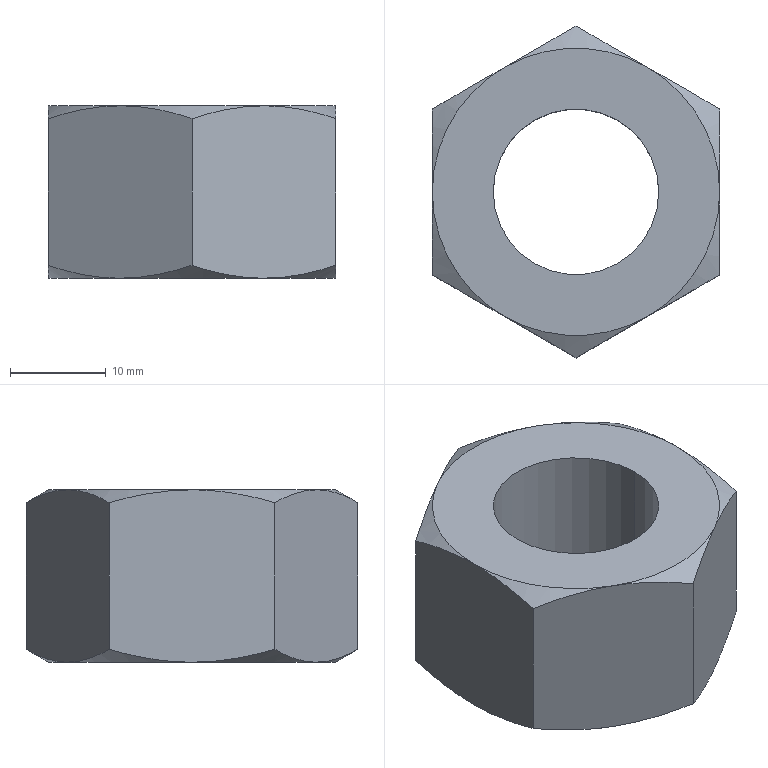Part | SolidWorks | features BaseBody 1 | 1 solid | 22 faces | box 30 x 34.641 x 18 mm | volume 9743 mm3 | cone 12 | plane 8 | cylinder 2 | commonest cylinder face diameters 17.294 x2
STEP:
#1=CARTESIAN_POINT('',(-8.647,0.,18.));
#2=VERTEX_POINT('',#1);
#3=CARTESIAN_POINT('',(8.647,0.,18.));
#4=VERTEX_POINT('',#3);
#5=CARTESIAN_POINT('',(0.,0.,18.));
#6=DIRECTION('',(0.,0.,1.));
#7=DIRECTION('',(1.,0.,0.));
#8=AXIS2_PLACEMENT_3D('',#5,#6,#7);
#9=CIRCLE('',#8,8.647);
#10=EDGE_CURVE('',#2,#4,#9,.T.);
#11=ORIENTED_EDGE('',*,*,#10,.T.);
#12=CARTESIAN_POINT('',(8.647,0.,0.));
#13=VERTEX_POINT('',#12);
#14=CARTESIAN_POINT('',(8.647,0.,18.));
#15=DIRECTION('',(0.,0.,-1.));
#16=VECTOR('',#15,1000.);
#17=LINE('',#14,#16);
#18=EDGE_CURVE('',#4,#13,#17,.T.);
#19=ORIENTED_EDGE('',*,*,#18,.T.);
#20=CARTESIAN_POINT('',(-8.647,0.,0.));
#21=VERTEX_POINT('',#20);
#22=CARTESIAN_POINT('',(0.,0.,0.));
#23=DIRECTION('',(0.,0.,1.));
#24=DIRECTION('',(1.,0.,0.));
#25=AXIS2_PLACEMENT_3D('',#22,#23,#24);
#26=CIRCLE('',#25,8.647);
#27=EDGE_CURVE('',#21,#13,#26,.T.);
#28=ORIENTED_EDGE('',*,*,#27,.F.);
#29=CARTESIAN_POINT('',(-8.647,0.,18.));
#30=DIRECTION('',(0.,0.,-1.));
#31=VECTOR('',#30,1000.);
#32=LINE('',#29,#31);
#33=EDGE_CURVE('',#2,#21,#32,.T.);
#34=ORIENTED_EDGE('',*,*,#33,.F.);
#35=EDGE_LOOP('',(#11,#19,#28,#34));
#36=FACE_OUTER_BOUND('',#35,.T.);
#37=CARTESIAN_POINT('',(0.,0.,18.));
#38=DIRECTION('',(0.,0.,-1.));
#39=DIRECTION('',(-1.,0.,0.));
#40=AXIS2_PLACEMENT_3D('',#37,#38,#39);
#41=CYLINDRICAL_SURFACE('',#40,8.647);
#42=ADVANCED_FACE('',(#36),#41,.F.);
#43=CARTESIAN_POINT('',(15.,8.66,16.66));
#44=VERTEX_POINT('',#43);
#45=CARTESIAN_POINT('',(7.5,12.99,18.));
#46=VERTEX_POINT('',#45);
#47=CARTESIAN_POINT('',(15.,8.66,16.66));
#48=CARTESIAN_POINT('',(13.773,9.369,17.069));
#49=CARTESIAN_POINT('',(12.537,10.082,17.406));
#50=CARTESIAN_POINT('',(10.04,11.524,17.872));
#51=CARTESIAN_POINT('',(8.778,12.253,18.));
#52=CARTESIAN_POINT('',(7.5,12.99,18.));
#53=B_SPLINE_CURVE_WITH_KNOTS('',3,(#47,#48,#49,#50,#51,#52),.UNSPECIFIED.,.F.,.F.,(4,2,4),(0.000000238,0.004382,0.008763),.UNSPECIFIED.);
#54=EDGE_CURVE('',#44,#46,#53,.T.);
#55=ORIENTED_EDGE('',*,*,#54,.F.);
#56=CARTESIAN_POINT('',(15.,8.66,1.34));
#57=VERTEX_POINT('',#56);
#58=CARTESIAN_POINT('',(15.,8.66,18.));
#59=DIRECTION('',(0.,0.,-1.));
#60=VECTOR('',#59,1000.);
#61=LINE('',#58,#60);
#62=EDGE_CURVE('',#44,#57,#61,.T.);
#63=ORIENTED_EDGE('',*,*,#62,.T.);
#64=CARTESIAN_POINT('',(7.5,12.99,0.));
#65=VERTEX_POINT('',#64);
#66=CARTESIAN_POINT('',(7.5,12.99,0.));
#67=CARTESIAN_POINT('',(8.136,12.623,0.));
#68=CARTESIAN_POINT('',(8.776,12.254,0.03167));
#69=CARTESIAN_POINT('',(10.041,11.524,0.1542));
#70=CARTESIAN_POINT('',(10.669,11.161,0.245));
#71=CARTESIAN_POINT('',(12.542,10.079,0.595));
#72=CARTESIAN_POINT('',(13.776,9.367,0.9318));
#73=CARTESIAN_POINT('',(15.,8.66,1.34));
#74=B_SPLINE_CURVE_WITH_KNOTS('',3,(#66,#67,#68,#69,#70,#71,#72,#73),.UNSPECIFIED.,.F.,.F.,(4,2,2,4),(0.008763,0.01095,0.01313,0.01749),.UNSPECIFIED.);
#75=EDGE_CURVE('',#65,#57,#74,.T.);
#76=ORIENTED_EDGE('',*,*,#75,.F.);
#77=CARTESIAN_POINT('',(0.,17.321,1.34));
#78=VERTEX_POINT('',#77);
#79=CARTESIAN_POINT('',(0.,17.321,1.34));
#80=CARTESIAN_POINT('',(1.227,16.612,0.9308));
#81=CARTESIAN_POINT('',(2.463,15.899,0.5939));
#82=CARTESIAN_POINT('',(4.96,14.457,0.1277));
#83=CARTESIAN_POINT('',(6.222,13.728,0.));
#84=CARTESIAN_POINT('',(7.5,12.99,0.));
#85=B_SPLINE_CURVE_WITH_KNOTS('',3,(#79,#80,#81,#82,#83,#84),.UNSPECIFIED.,.F.,.F.,(4,2,4),(0.000000238,0.004382,0.008763),.UNSPECIFIED.);
#86=EDGE_CURVE('',#78,#65,#85,.T.);
#87=ORIENTED_EDGE('',*,*,#86,.F.);
#88=CARTESIAN_POINT('',(0.,17.321,16.66));
#89=VERTEX_POINT('',#88);
#90=CARTESIAN_POINT('',(0.,17.321,18.));
#91=DIRECTION('',(0.,0.,-1.));
#92=VECTOR('',#91,1000.);
#93=LINE('',#90,#92);
#94=EDGE_CURVE('',#89,#78,#93,.T.);
#95=ORIENTED_EDGE('',*,*,#94,.F.);
#96=CARTESIAN_POINT('',(7.5,12.99,18.));
#97=CARTESIAN_POINT('',(6.864,13.358,18.));
#98=CARTESIAN_POINT('',(6.224,13.727,17.968));
#99=CARTESIAN_POINT('',(4.959,14.457,17.846));
#100=CARTESIAN_POINT('',(4.331,14.82,17.755));
#101=CARTESIAN_POINT('',(2.458,15.901,17.405));
#102=CARTESIAN_POINT('',(1.224,16.614,17.068));
#103=CARTESIAN_POINT('',(0.,17.321,16.66));
#104=B_SPLINE_CURVE_WITH_KNOTS('',3,(#96,#97,#98,#99,#100,#101,#102,#103),.UNSPECIFIED.,.F.,.F.,(4,2,2,4),(0.008763,0.01095,0.01313,0.01749),.UNSPECIFIED.);
#105=EDGE_CURVE('',#46,#89,#104,.T.);
#106=ORIENTED_EDGE('',*,*,#105,.F.);
#107=EDGE_LOOP('',(#55,#63,#76,#87,#95,#106));
#108=FACE_OUTER_BOUND('',#107,.T.);
#109=CARTESIAN_POINT('',(15.,8.66,18.));
#110=DIRECTION('',(-0.5,-0.866,0.));
#111=DIRECTION('',(0.866,-0.5,0.));
#112=AXIS2_PLACEMENT_3D('',#109,#110,#111);
#113=PLANE('',#112);
#114=ADVANCED_FACE('',(#108),#113,.F.);
#115=CARTESIAN_POINT('',(-7.5,12.99,18.));
#116=VERTEX_POINT('',#115);
#117=CARTESIAN_POINT('',(0.,17.321,16.66));
#118=CARTESIAN_POINT('',(-1.227,16.612,17.069));
#119=CARTESIAN_POINT('',(-2.463,15.899,17.406));
#120=CARTESIAN_POINT('',(-4.96,14.457,17.872));
#121=CARTESIAN_POINT('',(-6.222,13.728,18.));
#122=CARTESIAN_POINT('',(-7.5,12.99,18.));
#123=B_SPLINE_CURVE_WITH_KNOTS('',3,(#117,#118,#119,#120,#121,#122),.UNSPECIFIED.,.F.,.F.,(4,2,4),(0.000000238,0.004382,0.008763),.UNSPECIFIED.);
#124=EDGE_CURVE('',#89,#116,#123,.T.);
#125=ORIENTED_EDGE('',*,*,#124,.F.);
#126=ORIENTED_EDGE('',*,*,#94,.T.);
#127=CARTESIAN_POINT('',(-7.5,12.99,0.));
#128=VERTEX_POINT('',#127);
#129=CARTESIAN_POINT('',(-7.5,12.99,0.));
#130=CARTESIAN_POINT('',(-6.864,13.358,0.));
#131=CARTESIAN_POINT('',(-6.224,13.727,0.03167));
#132=CARTESIAN_POINT('',(-4.959,14.457,0.1542));
#133=CARTESIAN_POINT('',(-4.331,14.82,0.245));
#134=CARTESIAN_POINT('',(-2.458,15.901,0.595));
#135=CARTESIAN_POINT('',(-1.224,16.614,0.9318));
#136=CARTESIAN_POINT('',(0.,17.321,1.34));
#137=B_SPLINE_CURVE_WITH_KNOTS('',3,(#129,#130,#131,#132,#133,#134,#135,#136),.UNSPECIFIED.,.F.,.F.,(4,2,2,4),(0.008763,0.01095,0.01313,0.01749),.UNSPECIFIED.);
#138=EDGE_CURVE('',#128,#78,#137,.T.);
#139=ORIENTED_EDGE('',*,*,#138,.F.);
#140=CARTESIAN_POINT('',(-15.,8.66,1.34));
#141=VERTEX_POINT('',#140);
#142=CARTESIAN_POINT('',(-15.,8.66,1.34));
#143=CARTESIAN_POINT('',(-13.773,9.369,0.9308));
#144=CARTESIAN_POINT('',(-12.537,10.082,0.5939));
#145=CARTESIAN_POINT('',(-10.04,11.524,0.1277));
#146=CARTESIAN_POINT('',(-8.778,12.253,0.));
#147=CARTESIAN_POINT('',(-7.5,12.99,0.));
#148=B_SPLINE_CURVE_WITH_KNOTS('',3,(#142,#143,#144,#145,#146,#147),.UNSPECIFIED.,.F.,.F.,(4,2,4),(0.000000238,0.004382,0.008763),.UNSPECIFIED.);
#149=EDGE_CURVE('',#141,#128,#148,.T.);
#150=ORIENTED_EDGE('',*,*,#149,.F.);
#151=CARTESIAN_POINT('',(-15.,8.66,16.66));
#152=VERTEX_POINT('',#151);
#153=CARTESIAN_POINT('',(-15.,8.66,18.));
#154=DIRECTION('',(0.,0.,-1.));
#155=VECTOR('',#154,1000.);
#156=LINE('',#153,#155);
#157=EDGE_CURVE('',#152,#141,#156,.T.);
#158=ORIENTED_EDGE('',*,*,#157,.F.);
#159=CARTESIAN_POINT('',(-7.5,12.99,18.));
#160=CARTESIAN_POINT('',(-8.136,12.623,18.));
#161=CARTESIAN_POINT('',(-8.776,12.254,17.968));
#162=CARTESIAN_POINT('',(-10.041,11.524,17.846));
#163=CARTESIAN_POINT('',(-10.669,11.161,17.755));
#164=CARTESIAN_POINT('',(-12.542,10.079,17.405));
#165=CARTESIAN_POINT('',(-13.776,9.367,17.068));
#166=CARTESIAN_POINT('',(-15.,8.66,16.66));
#167=B_SPLINE_CURVE_WITH_KNOTS('',3,(#159,#160,#161,#162,#163,#164,#165,#166),.UNSPECIFIED.,.F.,.F.,(4,2,2,4),(0.008763,0.01095,0.01313,0.01749),.UNSPECIFIED.);
#168=EDGE_CURVE('',#116,#152,#167,.T.);
#169=ORIENTED_EDGE('',*,*,#168,.F.);
#170=EDGE_LOOP('',(#125,#126,#139,#150,#158,#169));
#171=FACE_OUTER_BOUND('',#170,.T.);
#172=CARTESIAN_POINT('',(0.,17.321,18.));
#173=DIRECTION('',(0.5,-0.866,0.));
#174=DIRECTION('',(0.866,0.5,0.));
#175=AXIS2_PLACEMENT_3D('',#172,#173,#174);
#176=PLANE('',#175);
#177=ADVANCED_FACE('',(#171),#176,.F.);
#178=CARTESIAN_POINT('',(-15.,0.,18.));
#179=VERTEX_POINT('',#178);
#180=CARTESIAN_POINT('',(-15.,8.66,16.66));
#181=CARTESIAN_POINT('',(-15.,7.26,17.065));
#182=CARTESIAN_POINT('',(-15.,5.841,17.401));
#183=CARTESIAN_POINT('',(-15.,3.673,17.753));
#184=CARTESIAN_POINT('',(-15.,2.944,17.845));
#185=CARTESIAN_POINT('',(-15.,1.469,17.969));
#186=CARTESIAN_POINT('',(-15.,0.7328,18.));
#187=CARTESIAN_POINT('',(-15.,0.,18.));
#188=B_SPLINE_CURVE_WITH_KNOTS('',3,(#180,#181,#182,#183,#184,#185,#186,#187),.UNSPECIFIED.,.F.,.F.,(4,2,2,4),(0.0493,0.05368,0.05587,0.05807),.UNSPECIFIED.);
#189=EDGE_CURVE('',#152,#179,#188,.T.);
#190=ORIENTED_EDGE('',*,*,#189,.F.);
#191=ORIENTED_EDGE('',*,*,#157,.T.);
#192=CARTESIAN_POINT('',(-15.,0.,0.));
#193=VERTEX_POINT('',#192);
#194=CARTESIAN_POINT('',(-15.,0.,0.));
#195=CARTESIAN_POINT('',(-15.,0.7328,0.));
#196=CARTESIAN_POINT('',(-15.,1.469,0.03124));
#197=CARTESIAN_POINT('',(-15.,2.944,0.1551));
#198=CARTESIAN_POINT('',(-15.,3.673,0.2469));
#199=CARTESIAN_POINT('',(-15.,5.841,0.5989));
#200=CARTESIAN_POINT('',(-15.,7.26,0.9354));
#201=CARTESIAN_POINT('',(-15.,8.66,1.34));
#202=B_SPLINE_CURVE_WITH_KNOTS('',3,(#194,#195,#196,#197,#198,#199,#200,#201),.UNSPECIFIED.,.F.,.F.,(4,2,2,4),(0.02463,0.02682,0.02901,0.0334),.UNSPECIFIED.);
#203=EDGE_CURVE('',#193,#141,#202,.T.);
#204=ORIENTED_EDGE('',*,*,#203,.F.);
#205=CARTESIAN_POINT('',(-15.,-8.66,1.34));
#206=VERTEX_POINT('',#205);
#207=CARTESIAN_POINT('',(-15.,-8.66,1.34));
#208=CARTESIAN_POINT('',(-15.,-7.251,0.9328));
#209=CARTESIAN_POINT('',(-15.,-5.808,0.592));
#210=CARTESIAN_POINT('',(-15.,-2.919,0.126));
#211=CARTESIAN_POINT('',(-15.,-1.465,0.));
#212=CARTESIAN_POINT('',(-15.,0.,0.));
#213=B_SPLINE_CURVE_WITH_KNOTS('',3,(#207,#208,#209,#210,#211,#212),.UNSPECIFIED.,.F.,.F.,(4,2,4),(0.01586,0.02025,0.02463),.UNSPECIFIED.);
#214=EDGE_CURVE('',#206,#193,#213,.T.);
#215=ORIENTED_EDGE('',*,*,#214,.F.);
#216=CARTESIAN_POINT('',(-15.,-8.66,16.66));
#217=VERTEX_POINT('',#216);
#218=CARTESIAN_POINT('',(-15.,-8.66,18.));
#219=DIRECTION('',(0.,0.,-1.));
#220=VECTOR('',#219,1000.);
#221=LINE('',#218,#220);
#222=EDGE_CURVE('',#217,#206,#221,.T.);
#223=ORIENTED_EDGE('',*,*,#222,.F.);
#224=CARTESIAN_POINT('',(-15.,0.,18.));
#225=CARTESIAN_POINT('',(-15.,-1.465,18.));
#226=CARTESIAN_POINT('',(-15.,-2.919,17.874));
#227=CARTESIAN_POINT('',(-15.,-5.808,17.408));
#228=CARTESIAN_POINT('',(-15.,-7.251,17.067));
#229=CARTESIAN_POINT('',(-15.,-8.66,16.66));
#230=B_SPLINE_CURVE_WITH_KNOTS('',3,(#224,#225,#226,#227,#228,#229),.UNSPECIFIED.,.F.,.F.,(4,2,4),(0.05807,0.06245,0.06683),.UNSPECIFIED.);
#231=EDGE_CURVE('',#179,#217,#230,.T.);
#232=ORIENTED_EDGE('',*,*,#231,.F.);
#233=EDGE_LOOP('',(#190,#191,#204,#215,#223,#232));
#234=FACE_OUTER_BOUND('',#233,.T.);
#235=CARTESIAN_POINT('',(-15.,8.66,18.));
#236=DIRECTION('',(1.,0.,0.));
#237=DIRECTION('',(0.,1.,0.));
#238=AXIS2_PLACEMENT_3D('',#235,#236,#237);
#239=PLANE('',#238);
#240=ADVANCED_FACE('',(#234),#239,.F.);
#241=CARTESIAN_POINT('',(-7.5,-12.99,18.));
#242=VERTEX_POINT('',#241);
#243=CARTESIAN_POINT('',(-15.,-8.66,16.66));
#244=CARTESIAN_POINT('',(-13.773,-9.369,17.069));
#245=CARTESIAN_POINT('',(-12.537,-10.082,17.406));
#246=CARTESIAN_POINT('',(-10.04,-11.524,17.872));
#247=CARTESIAN_POINT('',(-8.778,-12.253,18.));
#248=CARTESIAN_POINT('',(-7.5,-12.99,18.));
#249=B_SPLINE_CURVE_WITH_KNOTS('',3,(#243,#244,#245,#246,#247,#248),.UNSPECIFIED.,.F.,.F.,(4,2,4),(0.000000238,0.004382,0.008763),.UNSPECIFIED.);
#250=EDGE_CURVE('',#217,#242,#249,.T.);
#251=ORIENTED_EDGE('',*,*,#250,.F.);
#252=ORIENTED_EDGE('',*,*,#222,.T.);
#253=CARTESIAN_POINT('',(-7.5,-12.99,0.));
#254=VERTEX_POINT('',#253);
#255=CARTESIAN_POINT('',(-7.5,-12.99,0.));
#256=CARTESIAN_POINT('',(-8.136,-12.623,0.));
#257=CARTESIAN_POINT('',(-8.776,-12.254,0.03167));
#258=CARTESIAN_POINT('',(-10.041,-11.524,0.1542));
#259=CARTESIAN_POINT('',(-10.669,-11.161,0.245));
#260=CARTESIAN_POINT('',(-12.542,-10.079,0.595));
#261=CARTESIAN_POINT('',(-13.776,-9.367,0.9318));
#262=CARTESIAN_POINT('',(-15.,-8.66,1.34));
#263=B_SPLINE_CURVE_WITH_KNOTS('',3,(#255,#256,#257,#258,#259,#260,#261,#262),.UNSPECIFIED.,.F.,.F.,(4,2,2,4),(0.008763,0.01095,0.01313,0.01749),.UNSPECIFIED.);
#264=EDGE_CURVE('',#254,#206,#263,.T.);
#265=ORIENTED_EDGE('',*,*,#264,.F.);
#266=CARTESIAN_POINT('',(0.,-17.321,1.34));
#267=VERTEX_POINT('',#266);
#268=CARTESIAN_POINT('',(0.,-17.321,1.34));
#269=CARTESIAN_POINT('',(-1.227,-16.612,0.9308));
#270=CARTESIAN_POINT('',(-2.463,-15.899,0.5939));
#271=CARTESIAN_POINT('',(-4.96,-14.457,0.1277));
#272=CARTESIAN_POINT('',(-6.222,-13.728,0.));
#273=CARTESIAN_POINT('',(-7.5,-12.99,0.));
#274=B_SPLINE_CURVE_WITH_KNOTS('',3,(#268,#269,#270,#271,#272,#273),.UNSPECIFIED.,.F.,.F.,(4,2,4),(0.000000238,0.004382,0.008763),.UNSPECIFIED.);
#275=EDGE_CURVE('',#267,#254,#274,.T.);
#276=ORIENTED_EDGE('',*,*,#275,.F.);
#277=CARTESIAN_POINT('',(0.,-17.321,16.66));
#278=VERTEX_POINT('',#277);
#279=CARTESIAN_POINT('',(0.,-17.321,18.));
#280=DIRECTION('',(0.,0.,-1.));
#281=VECTOR('',#280,1000.);
#282=LINE('',#279,#281);
#283=EDGE_CURVE('',#278,#267,#282,.T.);
#284=ORIENTED_EDGE('',*,*,#283,.F.);
#285=CARTESIAN_POINT('',(-7.5,-12.99,18.));
#286=CARTESIAN_POINT('',(-6.864,-13.358,18.));
#287=CARTESIAN_POINT('',(-6.224,-13.727,17.968));
#288=CARTESIAN_POINT('',(-4.959,-14.457,17.846));
#289=CARTESIAN_POINT('',(-4.331,-14.82,17.755));
#290=CARTESIAN_POINT('',(-2.458,-15.901,17.405));
#291=CARTESIAN_POINT('',(-1.224,-16.614,17.068));
#292=CARTESIAN_POINT('',(0.,-17.321,16.66));
#293=B_SPLINE_CURVE_WITH_KNOTS('',3,(#285,#286,#287,#288,#289,#290,#291,#292),.UNSPECIFIED.,.F.,.F.,(4,2,2,4),(0.008763,0.01095,0.01313,0.01749),.UNSPECIFIED.);
#294=EDGE_CURVE('',#242,#278,#293,.T.);
#295=ORIENTED_EDGE('',*,*,#294,.F.);
#296=EDGE_LOOP('',(#251,#252,#265,#276,#284,#295));
#297=FACE_OUTER_BOUND('',#296,.T.);
#298=CARTESIAN_POINT('',(-15.,-8.66,18.));
#299=DIRECTION('',(0.5,0.866,0.));
#300=DIRECTION('',(-0.866,0.5,0.));
#301=AXIS2_PLACEMENT_3D('',#298,#299,#300);
#302=PLANE('',#301);
#303=ADVANCED_FACE('',(#297),#302,.F.);
#304=CARTESIAN_POINT('',(7.5,-12.99,18.));
#305=VERTEX_POINT('',#304);
#306=CARTESIAN_POINT('',(0.,-17.321,16.66));
#307=CARTESIAN_POINT('',(1.227,-16.612,17.069));
#308=CARTESIAN_POINT('',(2.463,-15.899,17.406));
#309=CARTESIAN_POINT('',(4.96,-14.457,17.872));
#310=CARTESIAN_POINT('',(6.222,-13.728,18.));
#311=CARTESIAN_POINT('',(7.5,-12.99,18.));
#312=B_SPLINE_CURVE_WITH_KNOTS('',3,(#306,#307,#308,#309,#310,#311),.UNSPECIFIED.,.F.,.F.,(4,2,4),(0.000000238,0.004382,0.008763),.UNSPECIFIED.);
#313=EDGE_CURVE('',#278,#305,#312,.T.);
#314=ORIENTED_EDGE('',*,*,#313,.F.);
#315=ORIENTED_EDGE('',*,*,#283,.T.);
#316=CARTESIAN_POINT('',(7.5,-12.99,0.));
#317=VERTEX_POINT('',#316);
#318=CARTESIAN_POINT('',(7.5,-12.99,0.));
#319=CARTESIAN_POINT('',(6.864,-13.358,0.));
#320=CARTESIAN_POINT('',(6.224,-13.727,0.03167));
#321=CARTESIAN_POINT('',(4.959,-14.457,0.1542));
#322=CARTESIAN_POINT('',(4.331,-14.82,0.245));
#323=CARTESIAN_POINT('',(2.458,-15.901,0.595));
#324=CARTESIAN_POINT('',(1.224,-16.614,0.9318));
#325=CARTESIAN_POINT('',(0.,-17.321,1.34));
#326=B_SPLINE_CURVE_WITH_KNOTS('',3,(#318,#319,#320,#321,#322,#323,#324,#325),.UNSPECIFIED.,.F.,.F.,(4,2,2,4),(0.008763,0.01095,0.01313,0.01749),.UNSPECIFIED.);
#327=EDGE_CURVE('',#317,#267,#326,.T.);
#328=ORIENTED_EDGE('',*,*,#327,.F.);
#329=CARTESIAN_POINT('',(15.,-8.66,1.34));
#330=VERTEX_POINT('',#329);
#331=CARTESIAN_POINT('',(15.,-8.66,1.34));
#332=CARTESIAN_POINT('',(13.773,-9.369,0.9308));
#333=CARTESIAN_POINT('',(12.537,-10.082,0.5939));
#334=CARTESIAN_POINT('',(10.04,-11.524,0.1277));
#335=CARTESIAN_POINT('',(8.778,-12.253,0.));
#336=CARTESIAN_POINT('',(7.5,-12.99,0.));
#337=B_SPLINE_CURVE_WITH_KNOTS('',3,(#331,#332,#333,#334,#335,#336),.UNSPECIFIED.,.F.,.F.,(4,2,4),(0.000000238,0.004382,0.008763),.UNSPECIFIED.);
#338=EDGE_CURVE('',#330,#317,#337,.T.);
#339=ORIENTED_EDGE('',*,*,#338,.F.);
#340=CARTESIAN_POINT('',(15.,-8.66,16.66));
#341=VERTEX_POINT('',#340);
#342=CARTESIAN_POINT('',(15.,-8.66,18.));
#343=DIRECTION('',(0.,0.,-1.));
#344=VECTOR('',#343,1000.);
#345=LINE('',#342,#344);
#346=EDGE_CURVE('',#341,#330,#345,.T.);
#347=ORIENTED_EDGE('',*,*,#346,.F.);
#348=CARTESIAN_POINT('',(7.5,-12.99,18.));
#349=CARTESIAN_POINT('',(8.136,-12.623,18.));
#350=CARTESIAN_POINT('',(8.776,-12.254,17.968));
#351=CARTESIAN_POINT('',(10.041,-11.524,17.846));
#352=CARTESIAN_POINT('',(10.669,-11.161,17.755));
#353=CARTESIAN_POINT('',(12.542,-10.079,17.405));
#354=CARTESIAN_POINT('',(13.776,-9.367,17.068));
#355=CARTESIAN_POINT('',(15.,-8.66,16.66));
#356=B_SPLINE_CURVE_WITH_KNOTS('',3,(#348,#349,#350,#351,#352,#353,#354,#355),.UNSPECIFIED.,.F.,.F.,(4,2,2,4),(0.008763,0.01095,0.01313,0.01749),.UNSPECIFIED.);
#357=EDGE_CURVE('',#305,#341,#356,.T.);
#358=ORIENTED_EDGE('',*,*,#357,.F.);
#359=EDGE_LOOP('',(#314,#315,#328,#339,#347,#358));
#360=FACE_OUTER_BOUND('',#359,.T.);
#361=CARTESIAN_POINT('',(0.,-17.321,18.));
#362=DIRECTION('',(-0.5,0.866,0.));
#363=DIRECTION('',(-0.866,-0.5,0.));
#364=AXIS2_PLACEMENT_3D('',#361,#362,#363);
#365=PLANE('',#364);
#366=ADVANCED_FACE('',(#360),#365,.F.);
#367=CARTESIAN_POINT('',(15.,0.,18.));
#368=VERTEX_POINT('',#367);
#369=CARTESIAN_POINT('',(15.,-8.66,16.66));
#370=CARTESIAN_POINT('',(15.,-7.251,17.067));
#371=CARTESIAN_POINT('',(15.,-5.808,17.408));
#372=CARTESIAN_POINT('',(15.,-2.919,17.874));
#373=CARTESIAN_POINT('',(15.,-1.465,18.));
#374=CARTESIAN_POINT('',(15.,0.,18.));
#375=B_SPLINE_CURVE_WITH_KNOTS('',3,(#369,#370,#371,#372,#373,#374),.UNSPECIFIED.,.F.,.F.,(4,2,4),(0.01586,0.02025,0.02463),.UNSPECIFIED.);
#376=EDGE_CURVE('',#341,#368,#375,.T.);
#377=ORIENTED_EDGE('',*,*,#376,.F.);
#378=ORIENTED_EDGE('',*,*,#346,.T.);
#379=CARTESIAN_POINT('',(15.,0.,0.));
#380=VERTEX_POINT('',#379);
#381=CARTESIAN_POINT('',(15.,0.,0.));
#382=CARTESIAN_POINT('',(15.,-1.465,0.));
#383=CARTESIAN_POINT('',(15.,-2.919,0.126));
#384=CARTESIAN_POINT('',(15.,-5.808,0.592));
#385=CARTESIAN_POINT('',(15.,-7.251,0.9328));
#386=CARTESIAN_POINT('',(15.,-8.66,1.34));
#387=B_SPLINE_CURVE_WITH_KNOTS('',3,(#381,#382,#383,#384,#385,#386),.UNSPECIFIED.,.F.,.F.,(4,2,4),(0.05807,0.06245,0.06683),.UNSPECIFIED.);
#388=EDGE_CURVE('',#380,#330,#387,.T.);
#389=ORIENTED_EDGE('',*,*,#388,.F.);
#390=CARTESIAN_POINT('',(15.,8.66,1.34));
#391=CARTESIAN_POINT('',(15.,7.26,0.9354));
#392=CARTESIAN_POINT('',(15.,5.841,0.5989));
#393=CARTESIAN_POINT('',(15.,3.673,0.2469));
#394=CARTESIAN_POINT('',(15.,2.944,0.1551));
#395=CARTESIAN_POINT('',(15.,1.469,0.03124));
#396=CARTESIAN_POINT('',(15.,0.7328,0.));
#397=CARTESIAN_POINT('',(15.,0.,0.));
#398=B_SPLINE_CURVE_WITH_KNOTS('',3,(#390,#391,#392,#393,#394,#395,#396,#397),.UNSPECIFIED.,.F.,.F.,(4,2,2,4),(0.0493,0.05368,0.05587,0.05807),.UNSPECIFIED.);
#399=EDGE_CURVE('',#57,#380,#398,.T.);
#400=ORIENTED_EDGE('',*,*,#399,.F.);
#401=ORIENTED_EDGE('',*,*,#62,.F.);
#402=CARTESIAN_POINT('',(15.,0.,18.));
#403=CARTESIAN_POINT('',(15.,0.7328,18.));
#404=CARTESIAN_POINT('',(15.,1.469,17.969));
#405=CARTESIAN_POINT('',(15.,2.944,17.845));
#406=CARTESIAN_POINT('',(15.,3.673,17.753));
#407=CARTESIAN_POINT('',(15.,5.841,17.401));
#408=CARTESIAN_POINT('',(15.,7.26,17.065));
#409=CARTESIAN_POINT('',(15.,8.66,16.66));
#410=B_SPLINE_CURVE_WITH_KNOTS('',3,(#402,#403,#404,#405,#406,#407,#408,#409),.UNSPECIFIED.,.F.,.F.,(4,2,2,4),(0.02463,0.02682,0.02901,0.0334),.UNSPECIFIED.);
#411=EDGE_CURVE('',#368,#44,#410,.T.);
#412=ORIENTED_EDGE('',*,*,#411,.F.);
#413=EDGE_LOOP('',(#377,#378,#389,#400,#401,#412));
#414=FACE_OUTER_BOUND('',#413,.T.);
#415=CARTESIAN_POINT('',(15.,-8.66,18.));
#416=DIRECTION('',(-1.,0.,0.));
#417=DIRECTION('',(0.,-1.,0.));
#418=AXIS2_PLACEMENT_3D('',#415,#416,#417);
#419=PLANE('',#418);
#420=ADVANCED_FACE('',(#414),#419,.F.);
#421=ORIENTED_EDGE('',*,*,#10,.F.);
#422=CARTESIAN_POINT('',(0.,0.,18.));
#423=DIRECTION('',(0.,0.,1.));
#424=DIRECTION('',(1.,0.,0.));
#425=AXIS2_PLACEMENT_3D('',#422,#423,#424);
#426=CIRCLE('',#425,8.647);
#427=EDGE_CURVE('',#4,#2,#426,.T.);
#428=ORIENTED_EDGE('',*,*,#427,.F.);
#429=EDGE_LOOP('',(#421,#428));
#430=FACE_BOUND('',#429,.T.);
#431=CARTESIAN_POINT('',(0.,0.,18.));
#432=DIRECTION('',(0.,0.,1.));
#433=DIRECTION('',(1.,0.,0.));
#434=AXIS2_PLACEMENT_3D('',#431,#432,#433);
#435=CIRCLE('',#434,15.);
#436=EDGE_CURVE('',#305,#368,#435,.T.);
#437=ORIENTED_EDGE('',*,*,#436,.T.);
#438=CARTESIAN_POINT('',(0.,0.,18.));
#439=DIRECTION('',(0.,0.,1.));
#440=DIRECTION('',(1.,0.,0.));
#441=AXIS2_PLACEMENT_3D('',#438,#439,#440);
#442=CIRCLE('',#441,15.);
#443=EDGE_CURVE('',#368,#46,#442,.T.);
#444=ORIENTED_EDGE('',*,*,#443,.T.);
#445=CARTESIAN_POINT('',(0.,0.,18.));
#446=DIRECTION('',(0.,0.,1.));
#447=DIRECTION('',(1.,0.,0.));
#448=AXIS2_PLACEMENT_3D('',#445,#446,#447);
#449=CIRCLE('',#448,15.);
#450=EDGE_CURVE('',#46,#116,#449,.T.);
#451=ORIENTED_EDGE('',*,*,#450,.T.);
#452=CARTESIAN_POINT('',(0.,0.,18.));
#453=DIRECTION('',(0.,0.,1.));
#454=DIRECTION('',(1.,0.,0.));
#455=AXIS2_PLACEMENT_3D('',#452,#453,#454);
#456=CIRCLE('',#455,15.);
#457=EDGE_CURVE('',#116,#179,#456,.T.);
#458=ORIENTED_EDGE('',*,*,#457,.T.);
#459=CARTESIAN_POINT('',(0.,0.,18.));
#460=DIRECTION('',(0.,0.,1.));
#461=DIRECTION('',(1.,0.,0.));
#462=AXIS2_PLACEMENT_3D('',#459,#460,#461);
#463=CIRCLE('',#462,15.);
#464=EDGE_CURVE('',#179,#242,#463,.T.);
#465=ORIENTED_EDGE('',*,*,#464,.T.);
#466=CARTESIAN_POINT('',(0.,0.,18.));
#467=DIRECTION('',(0.,0.,1.));
#468=DIRECTION('',(1.,0.,0.));
#469=AXIS2_PLACEMENT_3D('',#466,#467,#468);
#470=CIRCLE('',#469,15.);
#471=EDGE_CURVE('',#242,#305,#470,.T.);
#472=ORIENTED_EDGE('',*,*,#471,.T.);
#473=EDGE_LOOP('',(#437,#444,#451,#458,#465,#472));
#474=FACE_OUTER_BOUND('',#473,.T.);
#475=CARTESIAN_POINT('',(-15.,25.981,18.));
#476=DIRECTION('',(0.,0.,1.));
#477=DIRECTION('',(1.,0.,0.));
#478=AXIS2_PLACEMENT_3D('',#475,#476,#477);
#479=PLANE('',#478);
#480=ADVANCED_FACE('',(#430,#474),#479,.T.);
#481=ORIENTED_EDGE('',*,*,#27,.T.);
#482=CARTESIAN_POINT('',(0.,0.,0.));
#483=DIRECTION('',(0.,0.,1.));
#484=DIRECTION('',(1.,0.,0.));
#485=AXIS2_PLACEMENT_3D('',#482,#483,#484);
#486=CIRCLE('',#485,8.647);
#487=EDGE_CURVE('',#13,#21,#486,.T.);
#488=ORIENTED_EDGE('',*,*,#487,.T.);
#489=EDGE_LOOP('',(#481,#488));
#490=FACE_BOUND('',#489,.T.);
#491=CARTESIAN_POINT('',(0.,0.,0.));
#492=DIRECTION('',(0.,0.,-1.));
#493=DIRECTION('',(-1.,0.,0.));
#494=AXIS2_PLACEMENT_3D('',#491,#492,#493);
#495=CIRCLE('',#494,15.);
#496=EDGE_CURVE('',#65,#380,#495,.T.);
#497=ORIENTED_EDGE('',*,*,#496,.T.);
#498=CARTESIAN_POINT('',(0.,0.,0.));
#499=DIRECTION('',(0.,0.,-1.));
#500=DIRECTION('',(-1.,0.,0.));
#501=AXIS2_PLACEMENT_3D('',#498,#499,#500);
#502=CIRCLE('',#501,15.);
#503=EDGE_CURVE('',#380,#317,#502,.T.);
#504=ORIENTED_EDGE('',*,*,#503,.T.);
#505=CARTESIAN_POINT('',(0.,0.,0.));
#506=DIRECTION('',(0.,0.,-1.));
#507=DIRECTION('',(-1.,0.,0.));
#508=AXIS2_PLACEMENT_3D('',#505,#506,#507);
#509=CIRCLE('',#508,15.);
#510=EDGE_CURVE('',#317,#254,#509,.T.);
#511=ORIENTED_EDGE('',*,*,#510,.T.);
#512=CARTESIAN_POINT('',(0.,0.,0.));
#513=DIRECTION('',(0.,0.,-1.));
#514=DIRECTION('',(-1.,0.,0.));
#515=AXIS2_PLACEMENT_3D('',#512,#513,#514);
#516=CIRCLE('',#515,15.);
#517=EDGE_CURVE('',#254,#193,#516,.T.);
#518=ORIENTED_EDGE('',*,*,#517,.T.);
#519=CARTESIAN_POINT('',(0.,0.,0.));
#520=DIRECTION('',(0.,0.,-1.));
#521=DIRECTION('',(-1.,0.,0.));
#522=AXIS2_PLACEMENT_3D('',#519,#520,#521);
#523=CIRCLE('',#522,15.);
#524=EDGE_CURVE('',#193,#128,#523,.T.);
#525=ORIENTED_EDGE('',*,*,#524,.T.);
#526=CARTESIAN_POINT('',(0.,0.,0.));
#527=DIRECTION('',(0.,0.,-1.));
#528=DIRECTION('',(-1.,0.,0.));
#529=AXIS2_PLACEMENT_3D('',#526,#527,#528);
#530=CIRCLE('',#529,15.);
#531=EDGE_CURVE('',#128,#65,#530,.T.);
#532=ORIENTED_EDGE('',*,*,#531,.T.);
#533=EDGE_LOOP('',(#497,#504,#511,#518,#525,#532));
#534=FACE_OUTER_BOUND('',#533,.T.);
#535=CARTESIAN_POINT('',(-15.,25.981,0.));
#536=DIRECTION('',(0.,0.,1.));
#537=DIRECTION('',(1.,0.,0.));
#538=AXIS2_PLACEMENT_3D('',#535,#536,#537);
#539=PLANE('',#538);
#540=ADVANCED_FACE('',(#490,#534),#539,.F.);
#541=ORIENTED_EDGE('',*,*,#18,.F.);
#542=ORIENTED_EDGE('',*,*,#427,.T.);
#543=ORIENTED_EDGE('',*,*,#33,.T.);
#544=ORIENTED_EDGE('',*,*,#487,.F.);
#545=EDGE_LOOP('',(#541,#542,#543,#544));
#546=FACE_OUTER_BOUND('',#545,.T.);
#547=CARTESIAN_POINT('',(0.,0.,18.));
#548=DIRECTION('',(0.,0.,-1.));
#549=DIRECTION('',(-1.,0.,0.));
#550=AXIS2_PLACEMENT_3D('',#547,#548,#549);
#551=CYLINDRICAL_SURFACE('',#550,8.647);
#552=ADVANCED_FACE('',(#546),#551,.F.);
#553=ORIENTED_EDGE('',*,*,#338,.T.);
#554=ORIENTED_EDGE('',*,*,#503,.F.);
#555=ORIENTED_EDGE('',*,*,#388,.T.);
#556=EDGE_LOOP('',(#553,#554,#555));
#557=FACE_OUTER_BOUND('',#556,.T.);
#558=CARTESIAN_POINT('',(0.,0.,0.));
#559=DIRECTION('',(0.,0.,1.));
#560=DIRECTION('',(-1.,0.,0.));
#561=AXIS2_PLACEMENT_3D('',#558,#559,#560);
#562=CONICAL_SURFACE('',#561,15.,1.047);
#563=ADVANCED_FACE('',(#557),#562,.T.);
#564=ORIENTED_EDGE('',*,*,#75,.T.);
#565=ORIENTED_EDGE('',*,*,#399,.T.);
#566=ORIENTED_EDGE('',*,*,#496,.F.);
#567=EDGE_LOOP('',(#564,#565,#566));
#568=FACE_OUTER_BOUND('',#567,.T.);
#569=CARTESIAN_POINT('',(0.,0.,0.));
#570=DIRECTION('',(0.,0.,1.));
#571=DIRECTION('',(-1.,0.,0.));
#572=AXIS2_PLACEMENT_3D('',#569,#570,#571);
#573=CONICAL_SURFACE('',#572,15.,1.047);
#574=ADVANCED_FACE('',(#568),#573,.T.);
#575=ORIENTED_EDGE('',*,*,#275,.T.);
#576=ORIENTED_EDGE('',*,*,#510,.F.);
#577=ORIENTED_EDGE('',*,*,#327,.T.);
#578=EDGE_LOOP('',(#575,#576,#577));
#579=FACE_OUTER_BOUND('',#578,.T.);
#580=CARTESIAN_POINT('',(0.,0.,0.));
#581=DIRECTION('',(0.,0.,1.));
#582=DIRECTION('',(-1.,0.,0.));
#583=AXIS2_PLACEMENT_3D('',#580,#581,#582);
#584=CONICAL_SURFACE('',#583,15.,1.047);
#585=ADVANCED_FACE('',(#579),#584,.T.);
#586=ORIENTED_EDGE('',*,*,#214,.T.);
#587=ORIENTED_EDGE('',*,*,#517,.F.);
#588=ORIENTED_EDGE('',*,*,#264,.T.);
#589=EDGE_LOOP('',(#586,#587,#588));
#590=FACE_OUTER_BOUND('',#589,.T.);
#591=CARTESIAN_POINT('',(0.,0.,0.));
#592=DIRECTION('',(0.,0.,1.));
#593=DIRECTION('',(-1.,0.,0.));
#594=AXIS2_PLACEMENT_3D('',#591,#592,#593);
#595=CONICAL_SURFACE('',#594,15.,1.047);
#596=ADVANCED_FACE('',(#590),#595,.T.);
#597=ORIENTED_EDGE('',*,*,#203,.T.);
#598=ORIENTED_EDGE('',*,*,#149,.T.);
#599=ORIENTED_EDGE('',*,*,#524,.F.);
#600=EDGE_LOOP('',(#597,#598,#599));
#601=FACE_OUTER_BOUND('',#600,.T.);
#602=CARTESIAN_POINT('',(0.,0.,0.));
#603=DIRECTION('',(0.,0.,1.));
#604=DIRECTION('',(-1.,0.,0.));
#605=AXIS2_PLACEMENT_3D('',#602,#603,#604);
#606=CONICAL_SURFACE('',#605,15.,1.047);
#607=ADVANCED_FACE('',(#601),#606,.T.);
#608=ORIENTED_EDGE('',*,*,#138,.T.);
#609=ORIENTED_EDGE('',*,*,#86,.T.);
#610=ORIENTED_EDGE('',*,*,#531,.F.);
#611=EDGE_LOOP('',(#608,#609,#610));
#612=FACE_OUTER_BOUND('',#611,.T.);
#613=CARTESIAN_POINT('',(0.,0.,0.));
#614=DIRECTION('',(0.,0.,1.));
#615=DIRECTION('',(-1.,0.,0.));
#616=AXIS2_PLACEMENT_3D('',#613,#614,#615);
#617=CONICAL_SURFACE('',#616,15.,1.047);
#618=ADVANCED_FACE('',(#612),#617,.T.);
#619=ORIENTED_EDGE('',*,*,#357,.T.);
#620=ORIENTED_EDGE('',*,*,#376,.T.);
#621=ORIENTED_EDGE('',*,*,#436,.F.);
#622=EDGE_LOOP('',(#619,#620,#621));
#623=FACE_OUTER_BOUND('',#622,.T.);
#624=CARTESIAN_POINT('',(0.,0.,18.));
#625=DIRECTION('',(0.,0.,-1.));
#626=DIRECTION('',(1.,0.,0.));
#627=AXIS2_PLACEMENT_3D('',#624,#625,#626);
#628=CONICAL_SURFACE('',#627,15.,1.047);
#629=ADVANCED_FACE('',(#623),#628,.T.);
#630=ORIENTED_EDGE('',*,*,#294,.T.);
#631=ORIENTED_EDGE('',*,*,#313,.T.);
#632=ORIENTED_EDGE('',*,*,#471,.F.);
#633=EDGE_LOOP('',(#630,#631,#632));
#634=FACE_OUTER_BOUND('',#633,.T.);
#635=CARTESIAN_POINT('',(0.,0.,18.));
#636=DIRECTION('',(0.,0.,-1.));
#637=DIRECTION('',(1.,0.,0.));
#638=AXIS2_PLACEMENT_3D('',#635,#636,#637);
#639=CONICAL_SURFACE('',#638,15.,1.047);
#640=ADVANCED_FACE('',(#634),#639,.T.);
#641=ORIENTED_EDGE('',*,*,#231,.T.);
#642=ORIENTED_EDGE('',*,*,#250,.T.);
#643=ORIENTED_EDGE('',*,*,#464,.F.);
#644=EDGE_LOOP('',(#641,#642,#643));
#645=FACE_OUTER_BOUND('',#644,.T.);
#646=CARTESIAN_POINT('',(0.,0.,18.));
#647=DIRECTION('',(0.,0.,-1.));
#648=DIRECTION('',(1.,0.,0.));
#649=AXIS2_PLACEMENT_3D('',#646,#647,#648);
#650=CONICAL_SURFACE('',#649,15.,1.047);
#651=ADVANCED_FACE('',(#645),#650,.T.);
#652=ORIENTED_EDGE('',*,*,#168,.T.);
#653=ORIENTED_EDGE('',*,*,#189,.T.);
#654=ORIENTED_EDGE('',*,*,#457,.F.);
#655=EDGE_LOOP('',(#652,#653,#654));
#656=FACE_OUTER_BOUND('',#655,.T.);
#657=CARTESIAN_POINT('',(0.,0.,18.));
#658=DIRECTION('',(0.,0.,-1.));
#659=DIRECTION('',(1.,0.,0.));
#660=AXIS2_PLACEMENT_3D('',#657,#658,#659);
#661=CONICAL_SURFACE('',#660,15.,1.047);
#662=ADVANCED_FACE('',(#656),#661,.T.);
#663=ORIENTED_EDGE('',*,*,#105,.T.);
#664=ORIENTED_EDGE('',*,*,#124,.T.);
#665=ORIENTED_EDGE('',*,*,#450,.F.);
#666=EDGE_LOOP('',(#663,#664,#665));
#667=FACE_OUTER_BOUND('',#666,.T.);
#668=CARTESIAN_POINT('',(0.,0.,18.));
#669=DIRECTION('',(0.,0.,-1.));
#670=DIRECTION('',(1.,0.,0.));
#671=AXIS2_PLACEMENT_3D('',#668,#669,#670);
#672=CONICAL_SURFACE('',#671,15.,1.047);
#673=ADVANCED_FACE('',(#667),#672,.T.);
#674=ORIENTED_EDGE('',*,*,#54,.T.);
#675=ORIENTED_EDGE('',*,*,#443,.F.);
#676=ORIENTED_EDGE('',*,*,#411,.T.);
#677=EDGE_LOOP('',(#674,#675,#676));
#678=FACE_OUTER_BOUND('',#677,.T.);
#679=CARTESIAN_POINT('',(0.,0.,18.));
#680=DIRECTION('',(0.,0.,-1.));
#681=DIRECTION('',(1.,0.,0.));
#682=AXIS2_PLACEMENT_3D('',#679,#680,#681);
#683=CONICAL_SURFACE('',#682,15.,1.047);
#684=ADVANCED_FACE('',(#678),#683,.T.);
#685=CLOSED_SHELL('',(#42,#114,#177,#240,#303,#366,#420,#480,#540,#552,#563,#574,#585,#596,#607,#618,#629,#640,#651,#662,#673,#684));
#686=MANIFOLD_SOLID_BREP('',#685);
#687=CARTESIAN_POINT('',(0.,0.,0.));
#688=DIRECTION('',(0.,0.,1.));
#689=DIRECTION('',(1.,0.,0.));
#690=AXIS2_PLACEMENT_3D('',#687,#688,#689);
#691=(LENGTH_UNIT()NAMED_UNIT(*)SI_UNIT(.MILLI.,.METRE.));
#692=UNCERTAINTY_MEASURE_WITH_UNIT(LENGTH_MEASURE(0.00001),#691,'','');
#693=(NAMED_UNIT(*)PLANE_ANGLE_UNIT()SI_UNIT($,.RADIAN.));
#694=(NAMED_UNIT(*)SI_UNIT($,.STERADIAN.)SOLID_ANGLE_UNIT());
#695=(GEOMETRIC_REPRESENTATION_CONTEXT(3)GLOBAL_UNCERTAINTY_ASSIGNED_CONTEXT((#692))GLOBAL_UNIT_ASSIGNED_CONTEXT((#691,#693,#694))REPRESENTATION_CONTEXT('',''));
#696=ADVANCED_BREP_SHAPE_REPRESENTATION('',(#686,#690),#695);